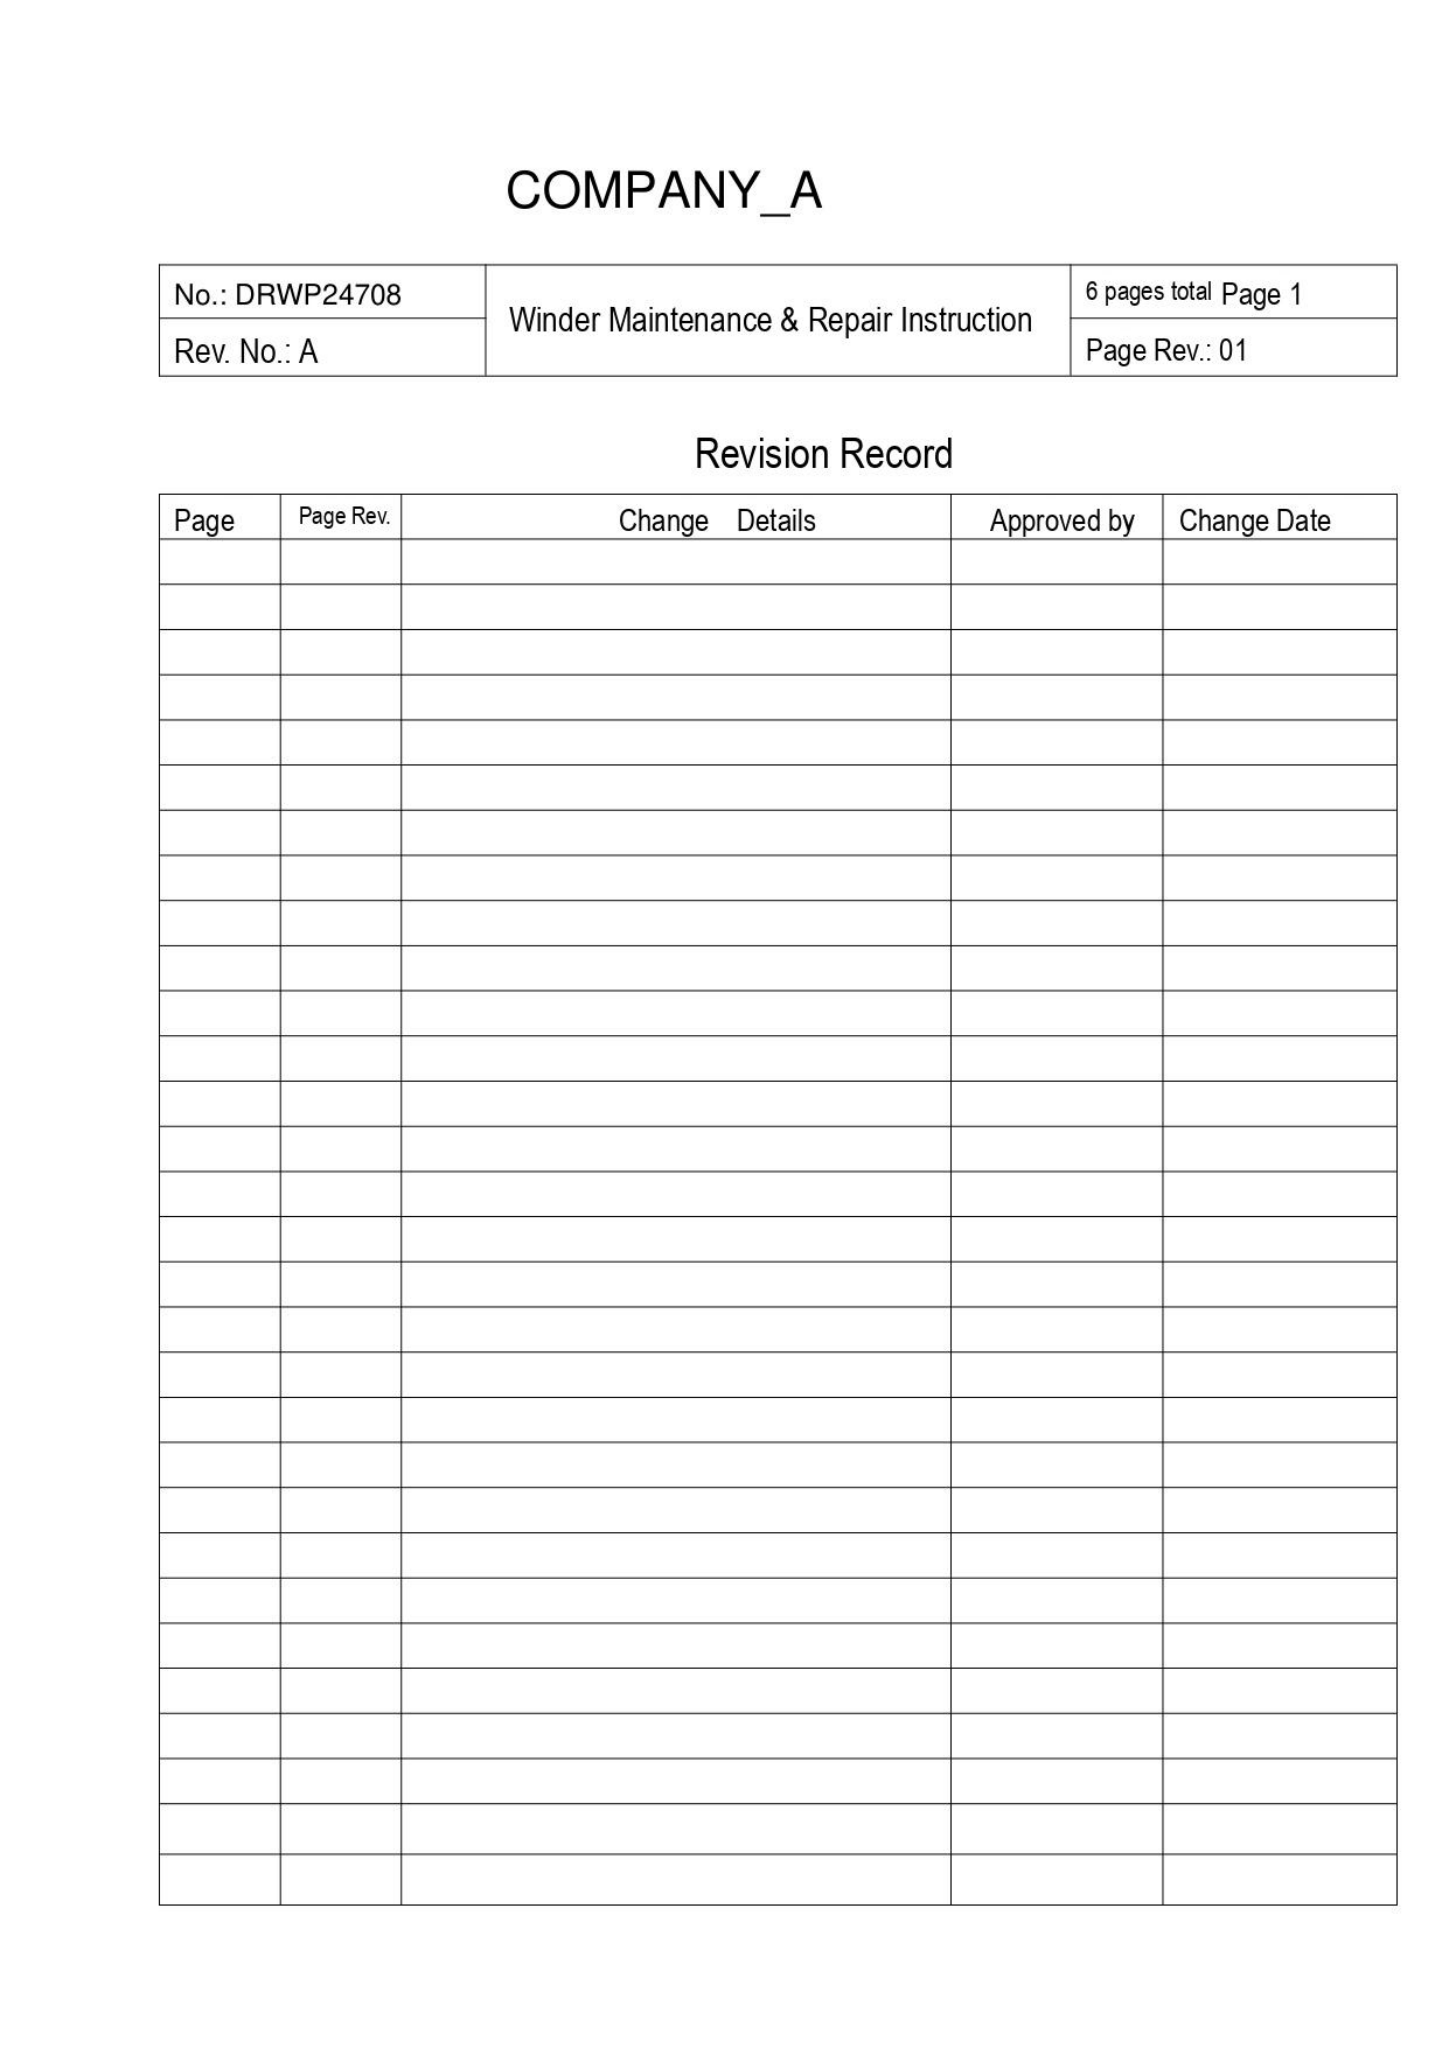COMPANY_A

| No.: DRWP24708 | Winder Maintenance & Repair Instruction | 6 pages total Page 1 |
|---|---|---|
| Rev. No.: A | | Page Rev.: 01 |

Revision Record

| Page | Page Rev. | Change Details | Approved by | Change Date |
|---|---|---|---|---|
| | | | | |
| | | | | |
| | | | | |
| | | | | |
| | | | | |
| | | | | |
| | | | | |
| | | | | |
| | | | | |
| | | | | |
| | | | | |
| | | | | |
| | | | | |
| | | | | |
| | | | | |
| | | | | |
| | | | | |
| | | | | |
| | | | | |
| | | | | |
| | | | | |
| | | | | |
| | | | | |
| | | | | |
| | | | | |
| | | | | |
| | | | | |
| | | | | |
| | | | | |
| | | | | |
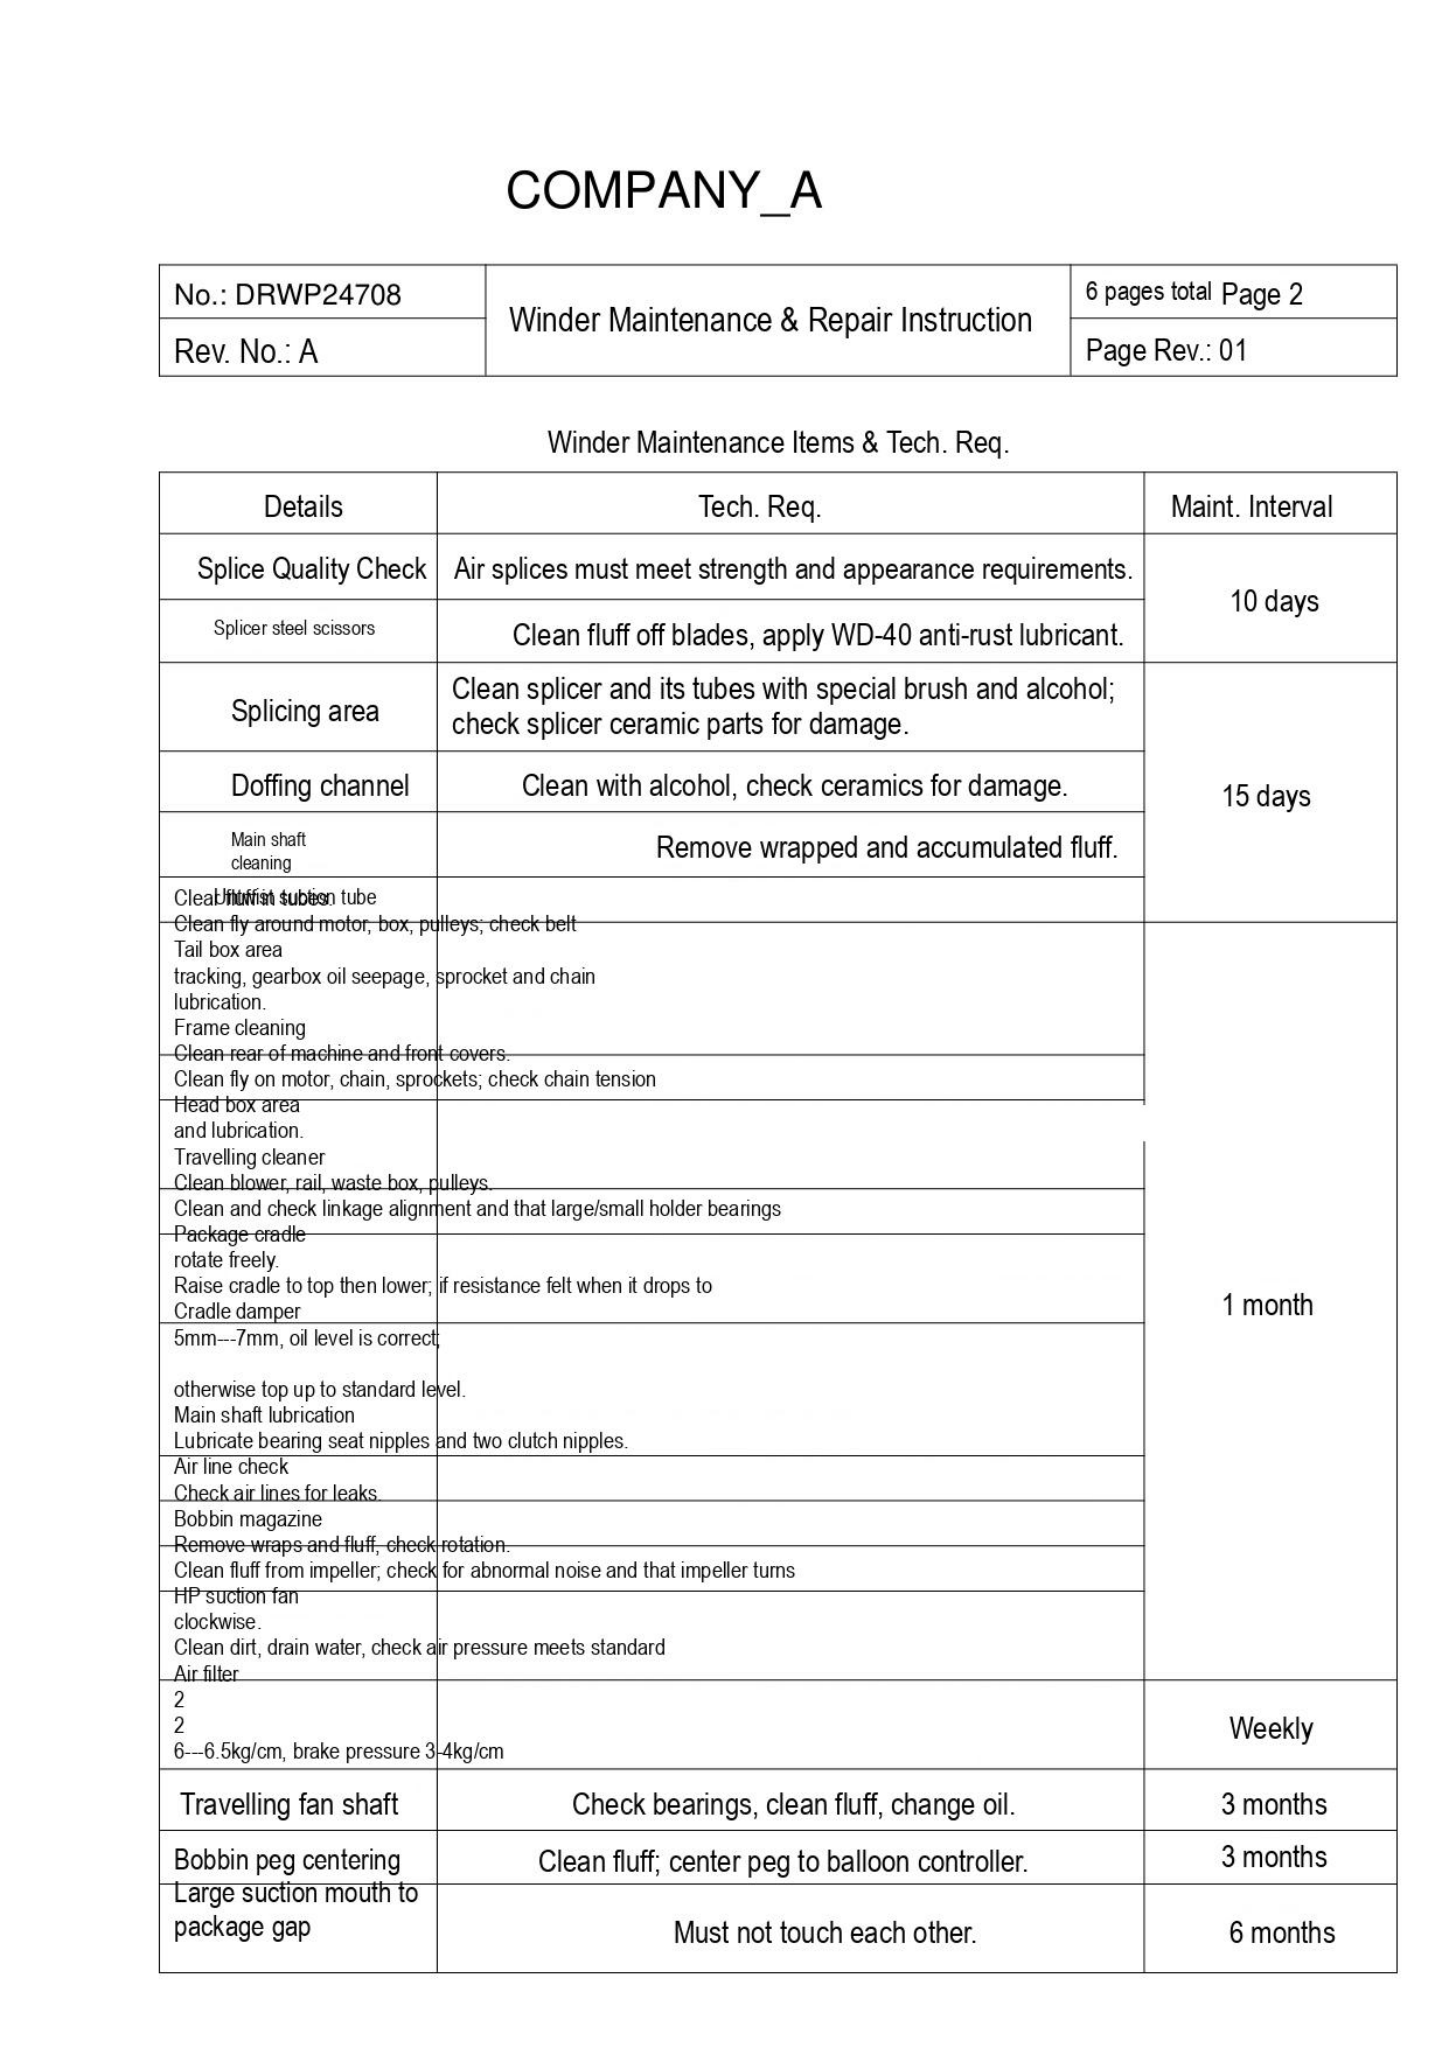# COMPANY_A

| No.: DRWP24708 | Winder Maintenance & Repair Instruction | 6 pages total Page 2 |
|---|---|---|
| Rev. No.: A | | Page Rev.: 01 |

Winder Maintenance Items & Tech. Req.

| Details | Tech. Req. | Maint. Interval |
|---|---|---|
| Splice Quality Check | Air splices must meet strength and appearance requirements. | 10 days |
| Splicer steel scissors | Clean fluff off blades, apply WD-40 anti-rust lubricant. | |
| Splicing area | Clean splicer and its tubes with special brush and alcohol; check splicer ceramic parts for damage. | 15 days |
| Doffing channel | Clean with alcohol, check ceramics for damage. | |
| Main shaft cleaning | Remove wrapped and accumulated fluff. | |
| Unfit suction tube | | |
| Clean fly around motor, box, pulleys; check belt<br>Tail box area<br>tracking, gearbox oil seepage, sprocket and chain<br>lubrication.<br>Frame cleaning | | 1 month |
| Clean rear of machine and front covers.<br>Clean fly on motor, chain, sprockets; check chain tension | | |
| Head box area<br>and lubrication.<br>Travelling cleaner | | |
| Clean blower, rail, waste box, pulleys.<br>Clean and check linkage alignment and that large/small holder bearings | | |
| Package cradle<br>rotate freely.<br>Raise cradle to top then lower; if resistance felt when it drops to<br>Cradle damper | | |
| 5mm---7mm, oil level is correct;<br><br>otherwise top up to standard level.<br>Main shaft lubrication<br>Lubricate bearing seat nipples and two clutch nipples. | | |
| Air line check<br>Check air lines for leaks. | | |
| Bobbin magazine<br>Remove wraps and fluff, check rotation. | | |
| Clean fluff from impeller; check for abnormal noise and that impeller turns | | |
| HP suction fan<br>clockwise.<br>Clean dirt, drain water, check air pressure meets standard<br>Air filter | | |
| 2<br>2<br>6---6.5kg/cm, brake pressure 3-4kg/cm | | Weekly |
| Travelling fan shaft | Check bearings, clean fluff, change oil. | 3 months |
| Bobbin peg centering | Clean fluff; center peg to balloon controller. | 3 months |
| Large suction mouth to package gap | Must not touch each other. | 6 months |
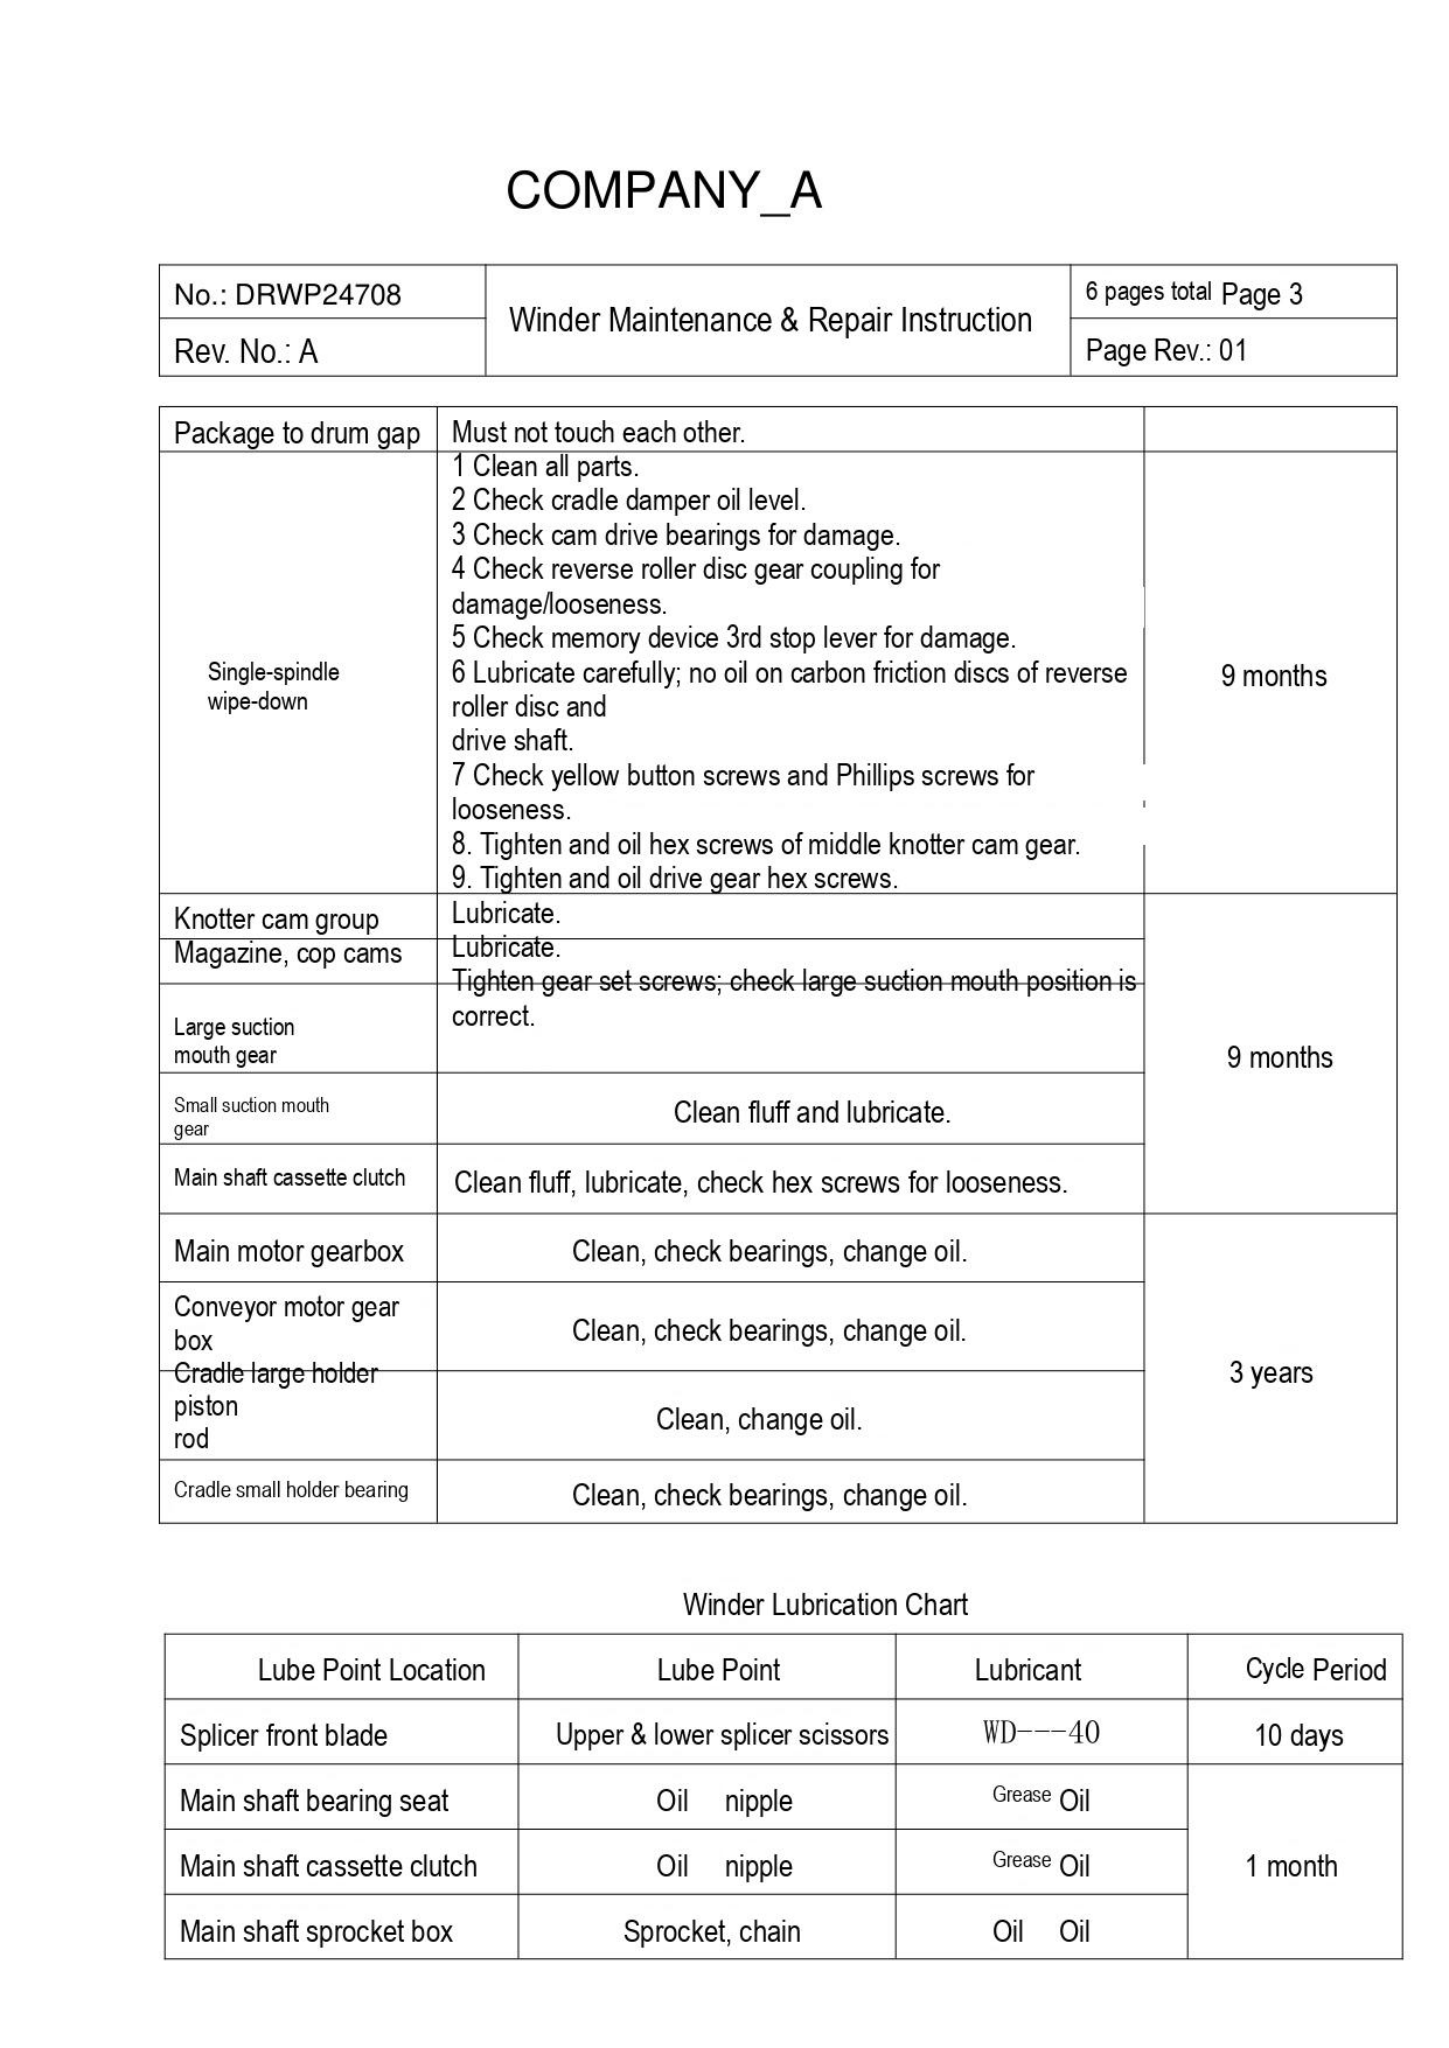COMPANY_A

| No.: DRWP24708 | Winder Maintenance & Repair Instruction | 6 pages total Page 3 |
|---|---|---|
| Rev. No.: A | | Page Rev.: 01 |

| Package to drum gap | Must not touch each other. | |
|---|---|---|
| Single-spindle wipe-down | 1 Clean all parts.<br>2 Check cradle damper oil level.<br>3 Check cam drive bearings for damage.<br>4 Check reverse roller disc gear coupling for damage/looseness.<br>5 Check memory device 3rd stop lever for damage.<br>6 Lubricate carefully; no oil on carbon friction discs of reverse roller disc and drive shaft.<br>7 Check yellow button screws and Phillips screws for looseness.<br>8. Tighten and oil hex screws of middle knotter cam gear.<br>9. Tighten and oil drive gear hex screws. | 9 months |
| Knotter cam group | Lubricate. | 9 months |
| Magazine, cop cams | Lubricate. | |
| Large suction mouth gear | Tighten gear set screws; check large suction mouth position is correct. | |
| Small suction mouth gear | Clean fluff and lubricate. | |
| Main shaft cassette clutch | Clean fluff, lubricate, check hex screws for looseness. | |
| Main motor gearbox | Clean, check bearings, change oil. | 3 years |
| Conveyor motor gear box | Clean, check bearings, change oil. | |
| Cradle large holder piston rod | Clean, change oil. | |
| Cradle small holder bearing | Clean, check bearings, change oil. | |

Winder Lubrication Chart

| Lube Point Location | Lube Point | Lubricant | Cycle Period |
|---|---|---|---|
| Splicer front blade | Upper & lower splicer scissors | WD---40 | 10 days |
| Main shaft bearing seat | Oil nipple | Grease Oil | 1 month |
| Main shaft cassette clutch | Oil nipple | Grease Oil | |
| Main shaft sprocket box | Sprocket, chain | Oil Oil | |
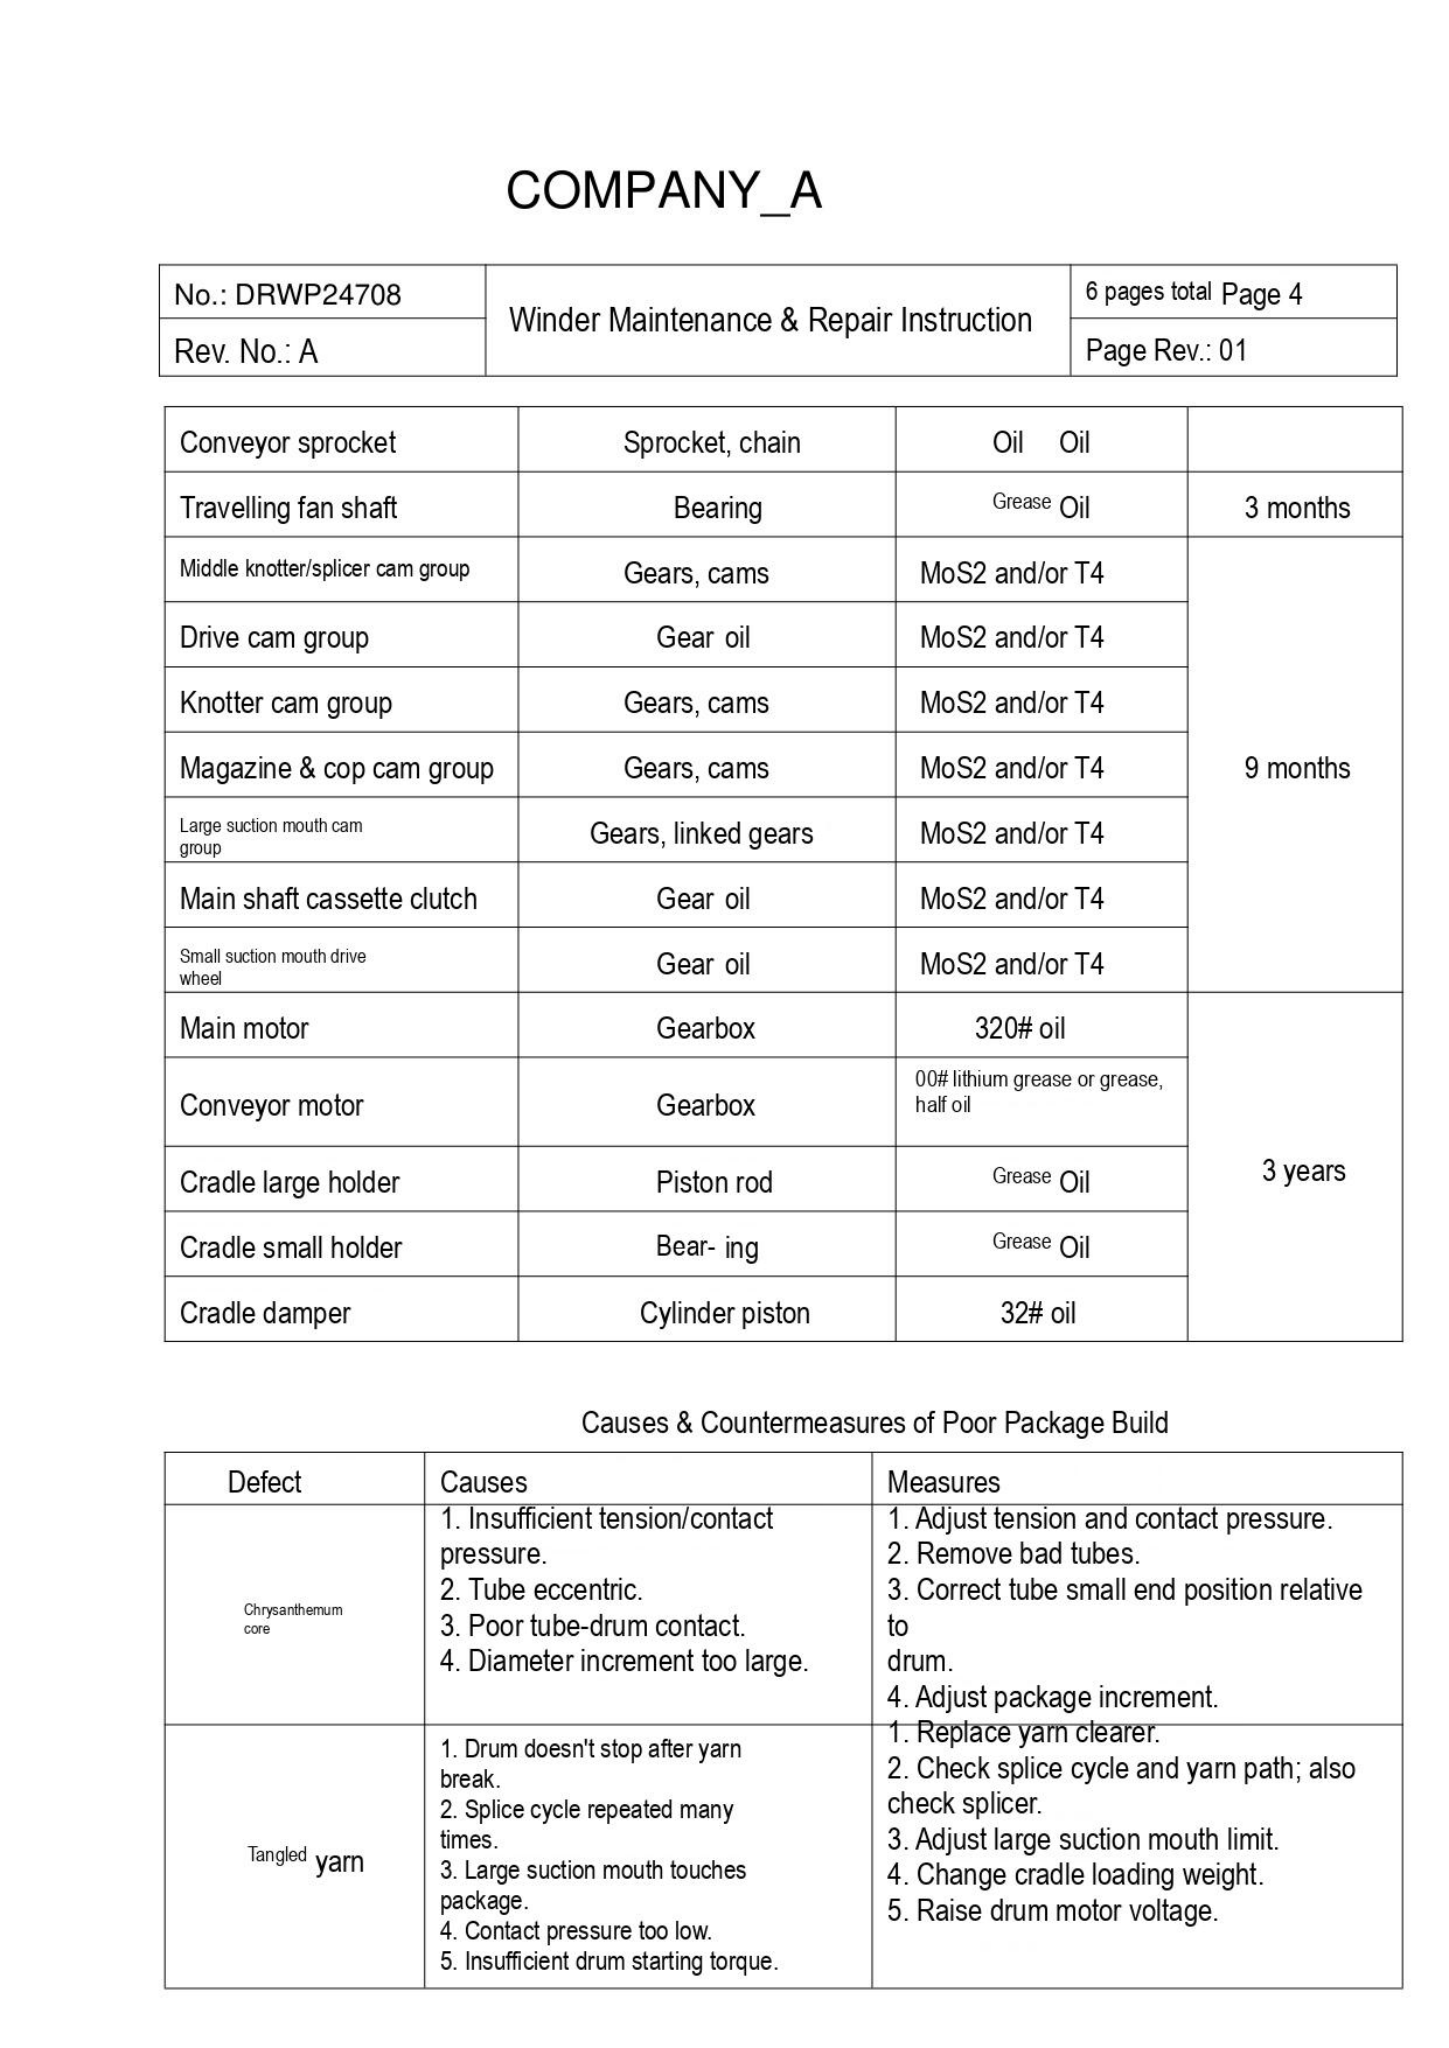COMPANY_A

| No.: DRWP24708 | Winder Maintenance & Repair Instruction | 6 pages total Page 4 |
|---|---|---|
| Rev. No.: A | | Page Rev.: 01 |

| Conveyor sprocket | Sprocket, chain | Oil Oil | |
|---|---|---|---|
| Travelling fan shaft | Bearing | Grease Oil | 3 months |
| Middle knotter/splicer cam group | Gears, cams | MoS2 and/or T4 | 9 months |
| Drive cam group | Gear oil | MoS2 and/or T4 | |
| Knotter cam group | Gears, cams | MoS2 and/or T4 | |
| Magazine & cop cam group | Gears, cams | MoS2 and/or T4 | |
| Large suction mouth cam group | Gears, linked gears | MoS2 and/or T4 | |
| Main shaft cassette clutch | Gear oil | MoS2 and/or T4 | |
| Small suction mouth drive wheel | Gear oil | MoS2 and/or T4 | |
| Main motor | Gearbox | 320# oil | 3 years |
| Conveyor motor | Gearbox | 00# lithium grease or grease, half oil | |
| Cradle large holder | Piston rod | Grease Oil | |
| Cradle small holder | Bear- ing | Grease Oil | |
| Cradle damper | Cylinder piston | 32# oil | |

Causes & Countermeasures of Poor Package Build

| Defect | Causes | Measures |
|---|---|---|
| Chrysanthemum core | 1. Insufficient tension/contact pressure.<br>2. Tube eccentric.<br>3. Poor tube-drum contact.<br>4. Diameter increment too large. | 1. Adjust tension and contact pressure.<br>2. Remove bad tubes.<br>3. Correct tube small end position relative to drum.<br>4. Adjust package increment. |
| Tangled yarn | 1. Drum doesn't stop after yarn break.<br>2. Splice cycle repeated many times.<br>3. Large suction mouth touches package.<br>4. Contact pressure too low.<br>5. Insufficient drum starting torque. | 1. Replace yarn clearer.<br>2. Check splice cycle and yarn path; also check splicer.<br>3. Adjust large suction mouth limit.<br>4. Change cradle loading weight.<br>5. Raise drum motor voltage. |
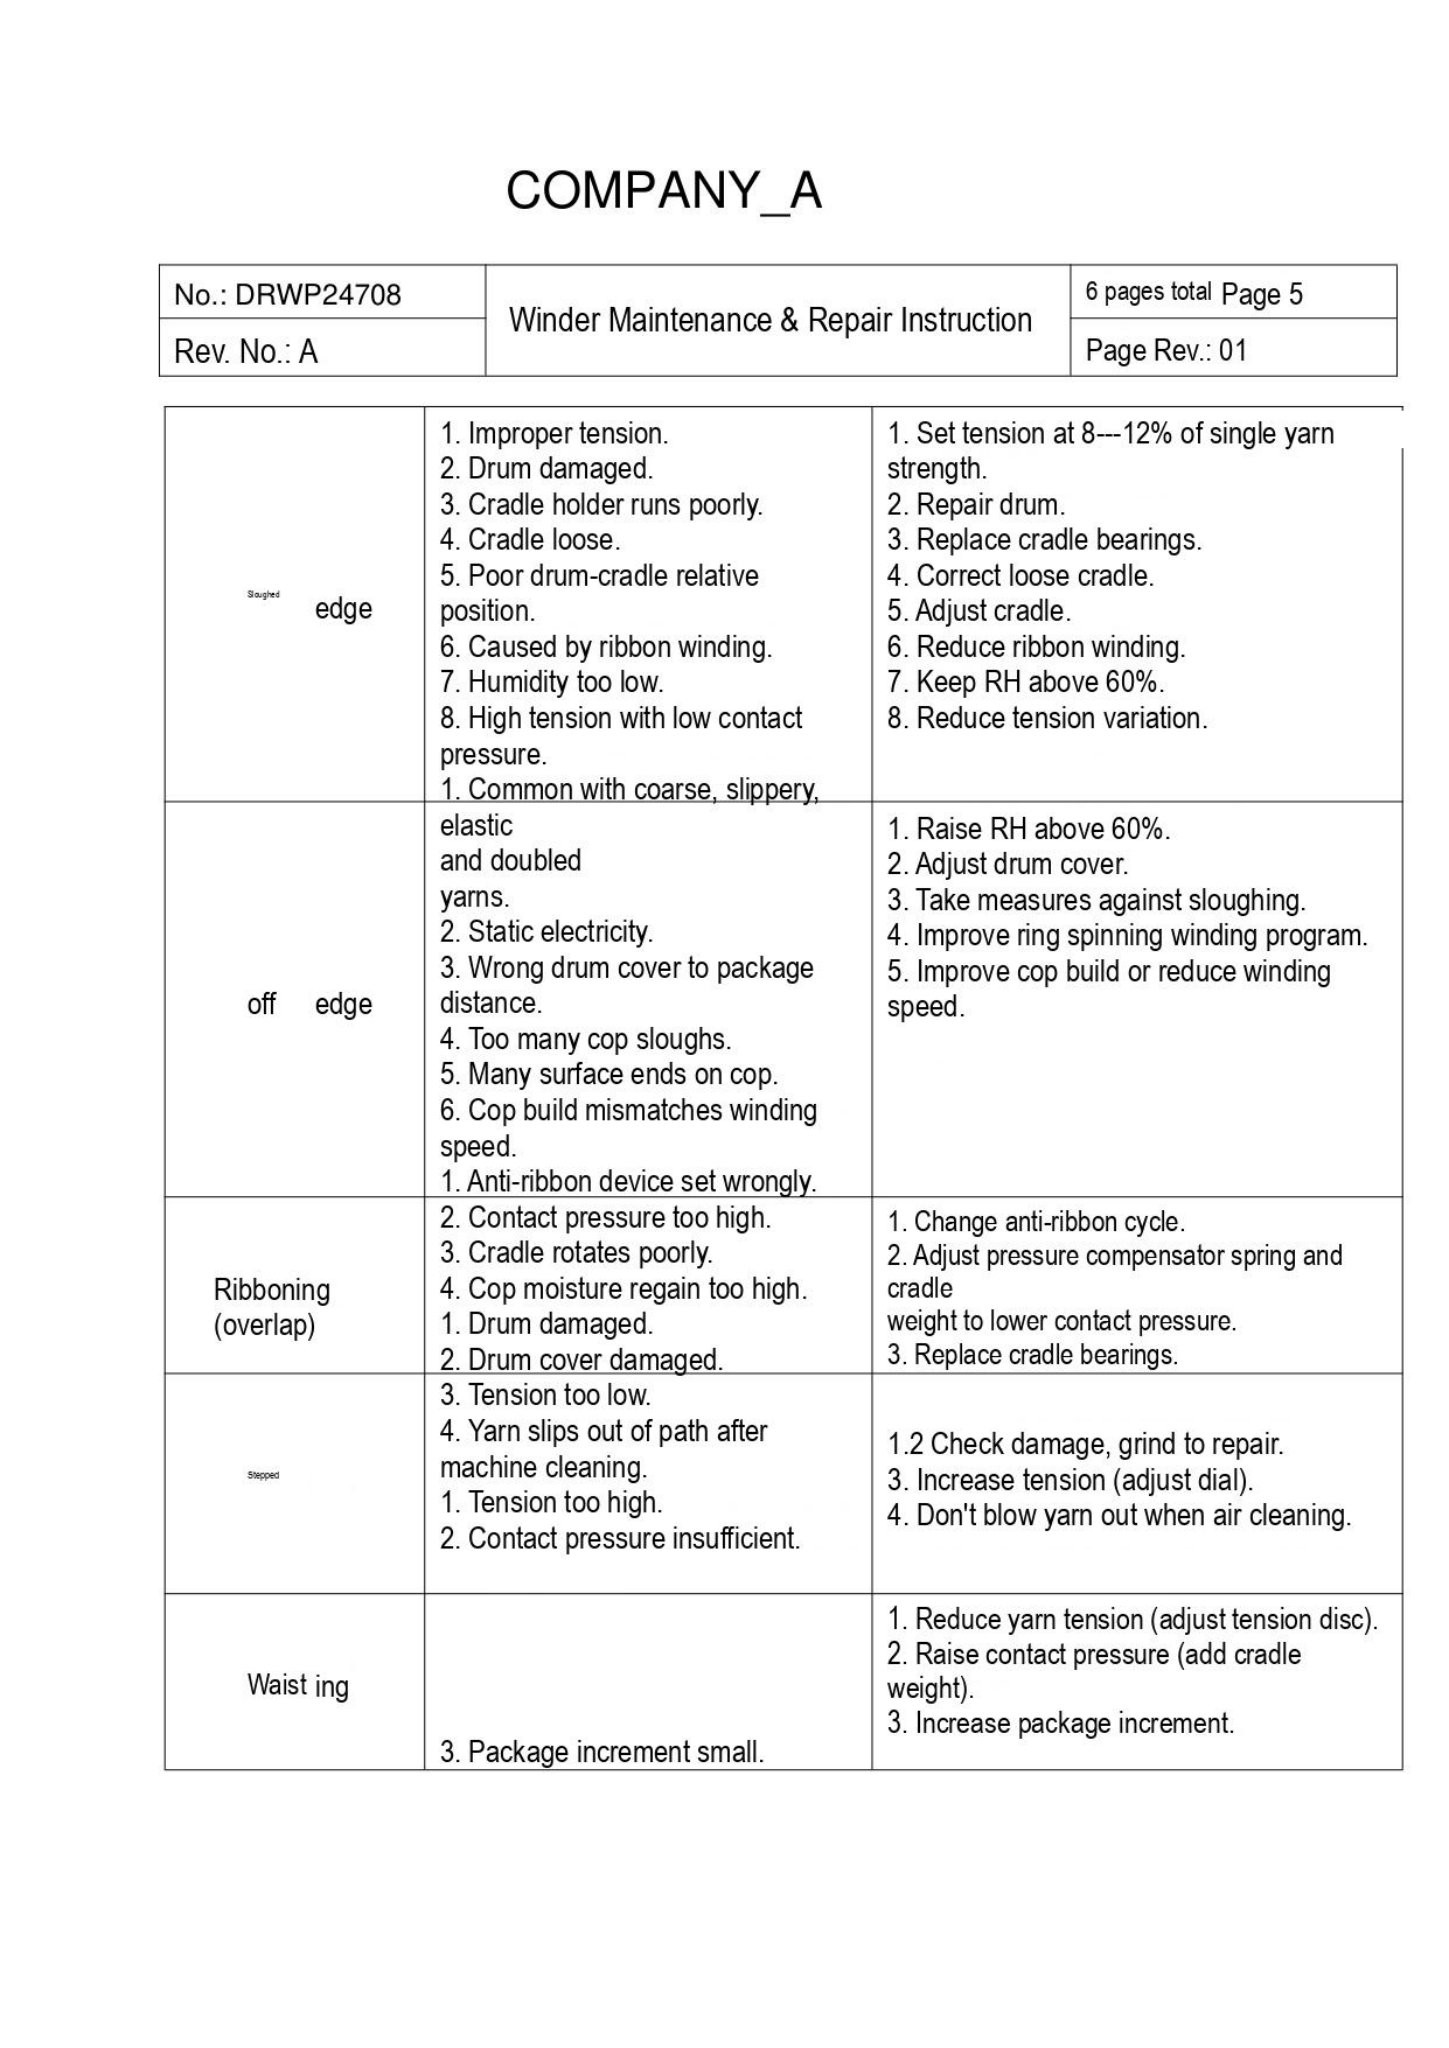COMPANY_A

| No.: DRWP24708 | Winder Maintenance & Repair Instruction | 6 pages total Page 5 |
|---|---|---|
| Rev. No.: A | | Page Rev.: 01 |

| | | |
|---|---|---|
| Sloughed edge | 1. Improper tension.<br>2. Drum damaged.<br>3. Cradle holder runs poorly.<br>4. Cradle loose.<br>5. Poor drum-cradle relative position.<br>6. Caused by ribbon winding.<br>7. Humidity too low.<br>8. High tension with low contact pressure.<br>1. Common with coarse, slippery, | 1. Set tension at 8---12% of single yarn strength.<br>2. Repair drum.<br>3. Replace cradle bearings.<br>4. Correct loose cradle.<br>5. Adjust cradle.<br>6. Reduce ribbon winding.<br>7. Keep RH above 60%.<br>8. Reduce tension variation. |
| off edge | elastic<br>and doubled<br>yarns.<br>2. Static electricity.<br>3. Wrong drum cover to package distance.<br>4. Too many cop sloughs.<br>5. Many surface ends on cop.<br>6. Cop build mismatches winding speed.<br>1. Anti-ribbon device set wrongly. | 1. Raise RH above 60%.<br>2. Adjust drum cover.<br>3. Take measures against sloughing.<br>4. Improve ring spinning winding program.<br>5. Improve cop build or reduce winding speed. |
| Ribboning (overlap) | 2. Contact pressure too high.<br>3. Cradle rotates poorly.<br>4. Cop moisture regain too high.<br>1. Drum damaged.<br>2. Drum cover damaged. | 1. Change anti-ribbon cycle.<br>2. Adjust pressure compensator spring and cradle<br>weight to lower contact pressure.<br>3. Replace cradle bearings. |
| Stepped | 3. Tension too low.<br>4. Yarn slips out of path after machine cleaning.<br>1. Tension too high.<br>2. Contact pressure insufficient. | 1.2 Check damage, grind to repair.<br>3. Increase tension (adjust dial).<br>4. Don't blow yarn out when air cleaning. |
| Waist ing | 3. Package increment small. | 1. Reduce yarn tension (adjust tension disc).<br>2. Raise contact pressure (add cradle weight).<br>3. Increase package increment. |
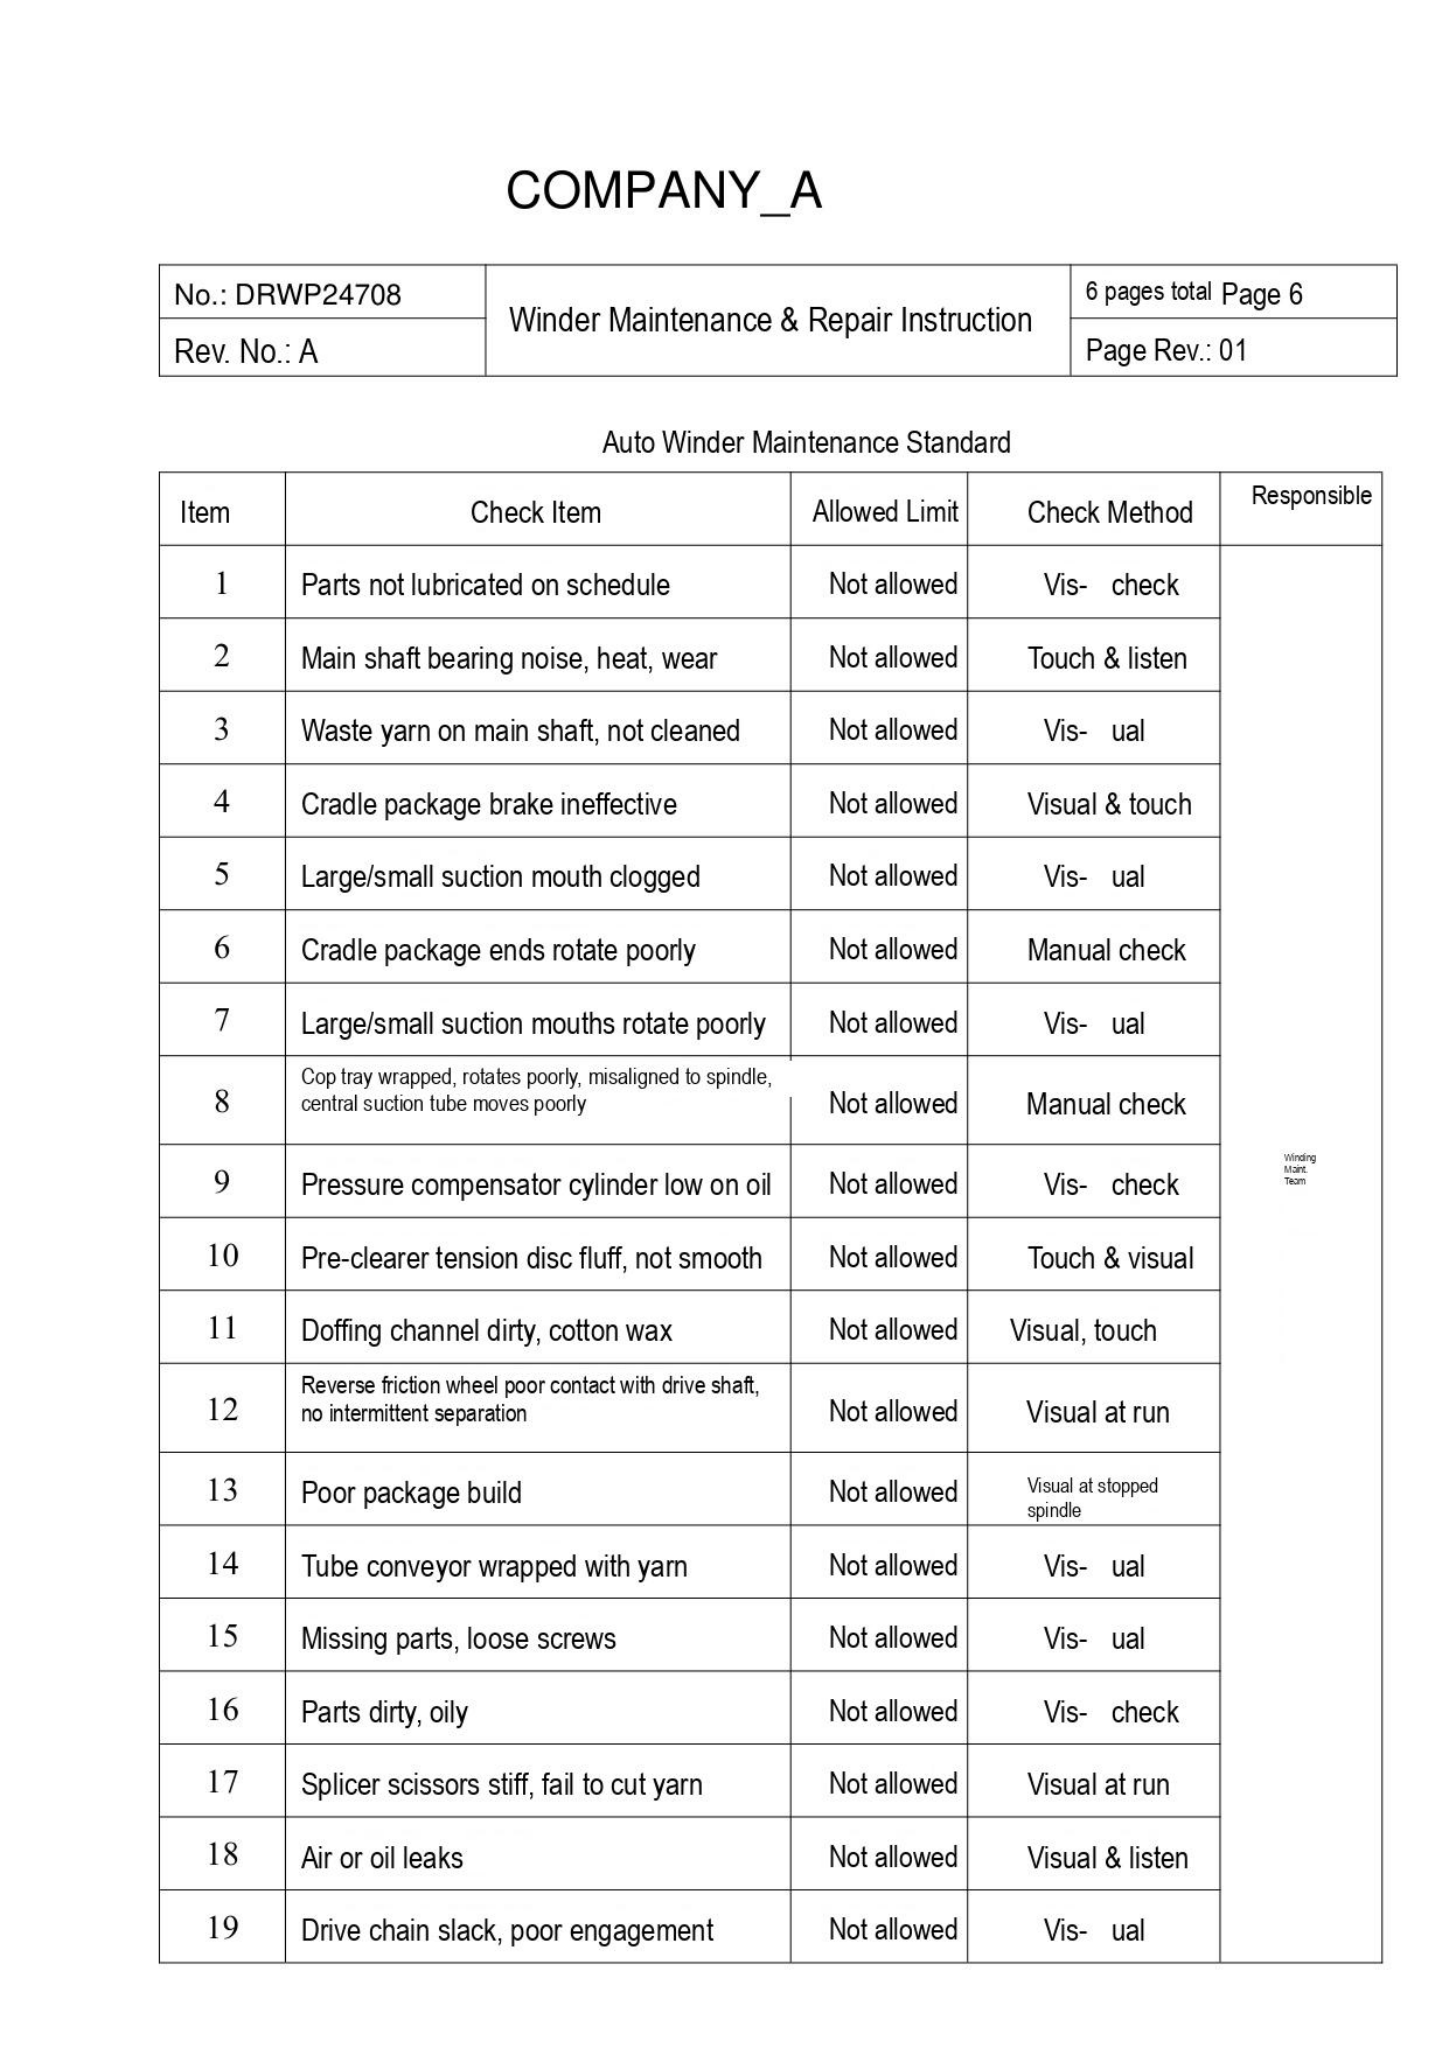COMPANY_A

| No.: DRWP24708 | Winder Maintenance & Repair Instruction | 6 pages total Page 6 |
|---|---|---|
| Rev. No.: A | | Page Rev.: 01 |

Auto Winder Maintenance Standard

| Item | Check Item | Allowed Limit | Check Method | Responsible |
|---|---|---|---|---|
| 1 | Parts not lubricated on schedule | Not allowed | Vis- check | Winding Maint. Team |
| 2 | Main shaft bearing noise, heat, wear | Not allowed | Touch & listen | |
| 3 | Waste yarn on main shaft, not cleaned | Not allowed | Vis- ual | |
| 4 | Cradle package brake ineffective | Not allowed | Visual & touch | |
| 5 | Large/small suction mouth clogged | Not allowed | Vis- ual | |
| 6 | Cradle package ends rotate poorly | Not allowed | Manual check | |
| 7 | Large/small suction mouths rotate poorly | Not allowed | Vis- ual | |
| 8 | Cop tray wrapped, rotates poorly, misaligned to spindle, central suction tube moves poorly | Not allowed | Manual check | |
| 9 | Pressure compensator cylinder low on oil | Not allowed | Vis- check | |
| 10 | Pre-clearer tension disc fluff, not smooth | Not allowed | Touch & visual | |
| 11 | Doffing channel dirty, cotton wax | Not allowed | Visual, touch | |
| 12 | Reverse friction wheel poor contact with drive shaft, no intermittent separation | Not allowed | Visual at run | |
| 13 | Poor package build | Not allowed | Visual at stopped spindle | |
| 14 | Tube conveyor wrapped with yarn | Not allowed | Vis- ual | |
| 15 | Missing parts, loose screws | Not allowed | Vis- ual | |
| 16 | Parts dirty, oily | Not allowed | Vis- check | |
| 17 | Splicer scissors stiff, fail to cut yarn | Not allowed | Visual at run | |
| 18 | Air or oil leaks | Not allowed | Visual & listen | |
| 19 | Drive chain slack, poor engagement | Not allowed | Vis- ual | |